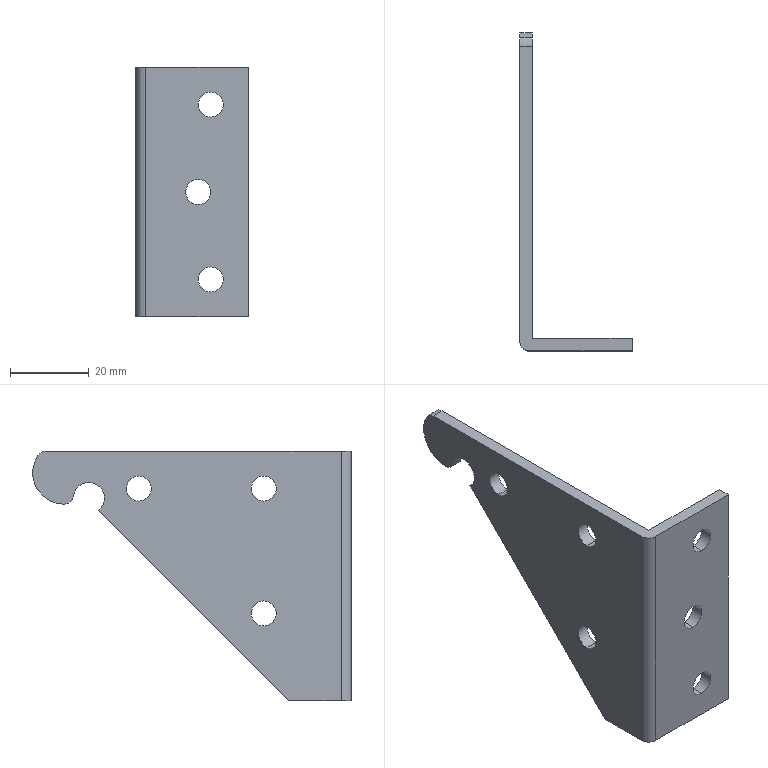Part | SolidWorks | features ICE 3, Extrusion 1 | 1 solid | 26 faces | box 28.575 x 80.975 x 63.5 mm | volume 14204 mm3 | cylinder 18 | plane 8 | commonest cylinder face diameters 6.35 x12 5.08 x4 7.925 x1 15.9 x1
STEP:
#1=CARTESIAN_POINT('',(15.875,0.,-50.8));
#2=VERTEX_POINT('',#1);
#3=CARTESIAN_POINT('',(15.875,0.,-57.15));
#4=VERTEX_POINT('',#3);
#5=CARTESIAN_POINT('',(15.875,0.,-53.975));
#6=DIRECTION('',(0.,-1.,0.));
#7=DIRECTION('',(0.,0.,-1.));
#8=AXIS2_PLACEMENT_3D('',#5,#6,#7);
#9=CIRCLE('',#8,3.175);
#10=EDGE_CURVE('',#2,#4,#9,.T.);
#11=ORIENTED_EDGE('',*,*,#10,.T.);
#12=CARTESIAN_POINT('',(15.875,3.175,-57.15));
#13=VERTEX_POINT('',#12);
#14=CARTESIAN_POINT('',(15.875,-22.225,-57.15));
#15=DIRECTION('',(0.,1.,0.));
#16=VECTOR('',#15,1000.);
#17=LINE('',#14,#16);
#18=EDGE_CURVE('',#4,#13,#17,.T.);
#19=ORIENTED_EDGE('',*,*,#18,.T.);
#20=CARTESIAN_POINT('',(15.875,3.175,-50.8));
#21=VERTEX_POINT('',#20);
#22=CARTESIAN_POINT('',(15.875,3.175,-53.975));
#23=DIRECTION('',(0.,1.,0.));
#24=DIRECTION('',(0.,0.,1.));
#25=AXIS2_PLACEMENT_3D('',#22,#23,#24);
#26=CIRCLE('',#25,3.175);
#27=EDGE_CURVE('',#13,#21,#26,.T.);
#28=ORIENTED_EDGE('',*,*,#27,.T.);
#29=CARTESIAN_POINT('',(15.875,-22.225,-50.8));
#30=DIRECTION('',(0.,1.,0.));
#31=VECTOR('',#30,1000.);
#32=LINE('',#29,#31);
#33=EDGE_CURVE('',#2,#21,#32,.T.);
#34=ORIENTED_EDGE('',*,*,#33,.F.);
#35=EDGE_LOOP('',(#11,#19,#28,#34));
#36=FACE_OUTER_BOUND('',#35,.T.);
#37=CARTESIAN_POINT('',(15.875,-22.225,-53.975));
#38=DIRECTION('',(0.,1.,0.));
#39=DIRECTION('',(0.,0.,1.));
#40=AXIS2_PLACEMENT_3D('',#37,#38,#39);
#41=CYLINDRICAL_SURFACE('',#40,3.175);
#42=ADVANCED_FACE('',(#36),#41,.F.);
#43=CARTESIAN_POINT('',(12.7,0.,-28.575));
#44=VERTEX_POINT('',#43);
#45=CARTESIAN_POINT('',(12.7,0.,-34.925));
#46=VERTEX_POINT('',#45);
#47=CARTESIAN_POINT('',(12.7,0.,-31.75));
#48=DIRECTION('',(0.,-1.,0.));
#49=DIRECTION('',(0.,0.,-1.));
#50=AXIS2_PLACEMENT_3D('',#47,#48,#49);
#51=CIRCLE('',#50,3.175);
#52=EDGE_CURVE('',#44,#46,#51,.T.);
#53=ORIENTED_EDGE('',*,*,#52,.T.);
#54=CARTESIAN_POINT('',(12.7,3.175,-34.925));
#55=VERTEX_POINT('',#54);
#56=CARTESIAN_POINT('',(12.7,-22.225,-34.925));
#57=DIRECTION('',(0.,1.,0.));
#58=VECTOR('',#57,1000.);
#59=LINE('',#56,#58);
#60=EDGE_CURVE('',#46,#55,#59,.T.);
#61=ORIENTED_EDGE('',*,*,#60,.T.);
#62=CARTESIAN_POINT('',(12.7,3.175,-28.575));
#63=VERTEX_POINT('',#62);
#64=CARTESIAN_POINT('',(12.7,3.175,-31.75));
#65=DIRECTION('',(0.,1.,0.));
#66=DIRECTION('',(0.,0.,1.));
#67=AXIS2_PLACEMENT_3D('',#64,#65,#66);
#68=CIRCLE('',#67,3.175);
#69=EDGE_CURVE('',#55,#63,#68,.T.);
#70=ORIENTED_EDGE('',*,*,#69,.T.);
#71=CARTESIAN_POINT('',(12.7,-22.225,-28.575));
#72=DIRECTION('',(0.,1.,0.));
#73=VECTOR('',#72,1000.);
#74=LINE('',#71,#73);
#75=EDGE_CURVE('',#44,#63,#74,.T.);
#76=ORIENTED_EDGE('',*,*,#75,.F.);
#77=EDGE_LOOP('',(#53,#61,#70,#76));
#78=FACE_OUTER_BOUND('',#77,.T.);
#79=CARTESIAN_POINT('',(12.7,-22.225,-31.75));
#80=DIRECTION('',(0.,1.,0.));
#81=DIRECTION('',(0.,0.,1.));
#82=AXIS2_PLACEMENT_3D('',#79,#80,#81);
#83=CYLINDRICAL_SURFACE('',#82,3.175);
#84=ADVANCED_FACE('',(#78),#83,.F.);
#85=CARTESIAN_POINT('',(15.875,0.,-6.35));
#86=VERTEX_POINT('',#85);
#87=CARTESIAN_POINT('',(15.875,0.,-12.7));
#88=VERTEX_POINT('',#87);
#89=CARTESIAN_POINT('',(15.875,0.,-9.525));
#90=DIRECTION('',(0.,-1.,0.));
#91=DIRECTION('',(0.,0.,-1.));
#92=AXIS2_PLACEMENT_3D('',#89,#90,#91);
#93=CIRCLE('',#92,3.175);
#94=EDGE_CURVE('',#86,#88,#93,.T.);
#95=ORIENTED_EDGE('',*,*,#94,.T.);
#96=CARTESIAN_POINT('',(15.875,3.175,-12.7));
#97=VERTEX_POINT('',#96);
#98=CARTESIAN_POINT('',(15.875,-22.225,-12.7));
#99=DIRECTION('',(0.,1.,0.));
#100=VECTOR('',#99,1000.);
#101=LINE('',#98,#100);
#102=EDGE_CURVE('',#88,#97,#101,.T.);
#103=ORIENTED_EDGE('',*,*,#102,.T.);
#104=CARTESIAN_POINT('',(15.875,3.175,-6.35));
#105=VERTEX_POINT('',#104);
#106=CARTESIAN_POINT('',(15.875,3.175,-9.525));
#107=DIRECTION('',(0.,1.,0.));
#108=DIRECTION('',(0.,0.,1.));
#109=AXIS2_PLACEMENT_3D('',#106,#107,#108);
#110=CIRCLE('',#109,3.175);
#111=EDGE_CURVE('',#97,#105,#110,.T.);
#112=ORIENTED_EDGE('',*,*,#111,.T.);
#113=CARTESIAN_POINT('',(15.875,-22.225,-6.35));
#114=DIRECTION('',(0.,1.,0.));
#115=VECTOR('',#114,1000.);
#116=LINE('',#113,#115);
#117=EDGE_CURVE('',#86,#105,#116,.T.);
#118=ORIENTED_EDGE('',*,*,#117,.F.);
#119=EDGE_LOOP('',(#95,#103,#112,#118));
#120=FACE_OUTER_BOUND('',#119,.T.);
#121=CARTESIAN_POINT('',(15.875,-22.225,-9.525));
#122=DIRECTION('',(0.,1.,0.));
#123=DIRECTION('',(0.,0.,1.));
#124=AXIS2_PLACEMENT_3D('',#121,#122,#123);
#125=CYLINDRICAL_SURFACE('',#124,3.175);
#126=ADVANCED_FACE('',(#120),#125,.F.);
#127=CARTESIAN_POINT('',(-3.175,53.975,-6.35));
#128=VERTEX_POINT('',#127);
#129=CARTESIAN_POINT('',(-3.175,53.975,-12.7));
#130=VERTEX_POINT('',#129);
#131=CARTESIAN_POINT('',(-3.175,53.975,-9.525));
#132=DIRECTION('',(1.,0.,0.));
#133=DIRECTION('',(0.,0.,-1.));
#134=AXIS2_PLACEMENT_3D('',#131,#132,#133);
#135=CIRCLE('',#134,3.175);
#136=EDGE_CURVE('',#128,#130,#135,.T.);
#137=ORIENTED_EDGE('',*,*,#136,.F.);
#138=CARTESIAN_POINT('',(0.,53.975,-6.35));
#139=VERTEX_POINT('',#138);
#140=CARTESIAN_POINT('',(-3.175,53.975,-6.35));
#141=DIRECTION('',(1.,0.,0.));
#142=VECTOR('',#141,1000.);
#143=LINE('',#140,#142);
#144=EDGE_CURVE('',#128,#139,#143,.T.);
#145=ORIENTED_EDGE('',*,*,#144,.T.);
#146=CARTESIAN_POINT('',(0.,53.975,-12.7));
#147=VERTEX_POINT('',#146);
#148=CARTESIAN_POINT('',(0.,53.975,-9.525));
#149=DIRECTION('',(1.,0.,0.));
#150=DIRECTION('',(0.,0.,-1.));
#151=AXIS2_PLACEMENT_3D('',#148,#149,#150);
#152=CIRCLE('',#151,3.175);
#153=EDGE_CURVE('',#139,#147,#152,.T.);
#154=ORIENTED_EDGE('',*,*,#153,.T.);
#155=CARTESIAN_POINT('',(-3.175,53.975,-12.7));
#156=DIRECTION('',(1.,0.,0.));
#157=VECTOR('',#156,1000.);
#158=LINE('',#155,#157);
#159=EDGE_CURVE('',#130,#147,#158,.T.);
#160=ORIENTED_EDGE('',*,*,#159,.F.);
#161=EDGE_LOOP('',(#137,#145,#154,#160));
#162=FACE_OUTER_BOUND('',#161,.T.);
#163=CARTESIAN_POINT('',(-3.175,53.975,-9.525));
#164=DIRECTION('',(1.,0.,0.));
#165=DIRECTION('',(0.,0.,-1.));
#166=AXIS2_PLACEMENT_3D('',#163,#164,#165);
#167=CYLINDRICAL_SURFACE('',#166,3.175);
#168=ADVANCED_FACE('',(#162),#167,.F.);
#169=CARTESIAN_POINT('',(-3.175,22.225,-38.1));
#170=VERTEX_POINT('',#169);
#171=CARTESIAN_POINT('',(-3.175,22.225,-44.45));
#172=VERTEX_POINT('',#171);
#173=CARTESIAN_POINT('',(-3.175,22.225,-41.275));
#174=DIRECTION('',(1.,0.,0.));
#175=DIRECTION('',(0.,0.,-1.));
#176=AXIS2_PLACEMENT_3D('',#173,#174,#175);
#177=CIRCLE('',#176,3.175);
#178=EDGE_CURVE('',#170,#172,#177,.T.);
#179=ORIENTED_EDGE('',*,*,#178,.F.);
#180=CARTESIAN_POINT('',(0.,22.225,-38.1));
#181=VERTEX_POINT('',#180);
#182=CARTESIAN_POINT('',(-3.175,22.225,-38.1));
#183=DIRECTION('',(1.,0.,0.));
#184=VECTOR('',#183,1000.);
#185=LINE('',#182,#184);
#186=EDGE_CURVE('',#170,#181,#185,.T.);
#187=ORIENTED_EDGE('',*,*,#186,.T.);
#188=CARTESIAN_POINT('',(0.,22.225,-44.45));
#189=VERTEX_POINT('',#188);
#190=CARTESIAN_POINT('',(0.,22.225,-41.275));
#191=DIRECTION('',(1.,0.,0.));
#192=DIRECTION('',(0.,0.,-1.));
#193=AXIS2_PLACEMENT_3D('',#190,#191,#192);
#194=CIRCLE('',#193,3.175);
#195=EDGE_CURVE('',#181,#189,#194,.T.);
#196=ORIENTED_EDGE('',*,*,#195,.T.);
#197=CARTESIAN_POINT('',(-3.175,22.225,-44.45));
#198=DIRECTION('',(1.,0.,0.));
#199=VECTOR('',#198,1000.);
#200=LINE('',#197,#199);
#201=EDGE_CURVE('',#172,#189,#200,.T.);
#202=ORIENTED_EDGE('',*,*,#201,.F.);
#203=EDGE_LOOP('',(#179,#187,#196,#202));
#204=FACE_OUTER_BOUND('',#203,.T.);
#205=CARTESIAN_POINT('',(-3.175,22.225,-41.275));
#206=DIRECTION('',(1.,0.,0.));
#207=DIRECTION('',(0.,0.,-1.));
#208=AXIS2_PLACEMENT_3D('',#205,#206,#207);
#209=CYLINDRICAL_SURFACE('',#208,3.175);
#210=ADVANCED_FACE('',(#204),#209,.F.);
#211=CARTESIAN_POINT('',(-3.175,22.225,-6.35));
#212=VERTEX_POINT('',#211);
#213=CARTESIAN_POINT('',(-3.175,22.225,-12.7));
#214=VERTEX_POINT('',#213);
#215=CARTESIAN_POINT('',(-3.175,22.225,-9.525));
#216=DIRECTION('',(1.,0.,0.));
#217=DIRECTION('',(0.,0.,-1.));
#218=AXIS2_PLACEMENT_3D('',#215,#216,#217);
#219=CIRCLE('',#218,3.175);
#220=EDGE_CURVE('',#212,#214,#219,.T.);
#221=ORIENTED_EDGE('',*,*,#220,.F.);
#222=CARTESIAN_POINT('',(0.,22.225,-6.35));
#223=VERTEX_POINT('',#222);
#224=CARTESIAN_POINT('',(-3.175,22.225,-6.35));
#225=DIRECTION('',(1.,0.,0.));
#226=VECTOR('',#225,1000.);
#227=LINE('',#224,#226);
#228=EDGE_CURVE('',#212,#223,#227,.T.);
#229=ORIENTED_EDGE('',*,*,#228,.T.);
#230=CARTESIAN_POINT('',(0.,22.225,-12.7));
#231=VERTEX_POINT('',#230);
#232=CARTESIAN_POINT('',(0.,22.225,-9.525));
#233=DIRECTION('',(1.,0.,0.));
#234=DIRECTION('',(0.,0.,-1.));
#235=AXIS2_PLACEMENT_3D('',#232,#233,#234);
#236=CIRCLE('',#235,3.175);
#237=EDGE_CURVE('',#223,#231,#236,.T.);
#238=ORIENTED_EDGE('',*,*,#237,.T.);
#239=CARTESIAN_POINT('',(-3.175,22.225,-12.7));
#240=DIRECTION('',(1.,0.,0.));
#241=VECTOR('',#240,1000.);
#242=LINE('',#239,#241);
#243=EDGE_CURVE('',#214,#231,#242,.T.);
#244=ORIENTED_EDGE('',*,*,#243,.F.);
#245=EDGE_LOOP('',(#221,#229,#238,#244));
#246=FACE_OUTER_BOUND('',#245,.T.);
#247=CARTESIAN_POINT('',(-3.175,22.225,-9.525));
#248=DIRECTION('',(1.,0.,0.));
#249=DIRECTION('',(0.,0.,-1.));
#250=AXIS2_PLACEMENT_3D('',#247,#248,#249);
#251=CYLINDRICAL_SURFACE('',#250,3.175);
#252=ADVANCED_FACE('',(#246),#251,.F.);
#253=CARTESIAN_POINT('',(-3.175,73.109,-13.512));
#254=VERTEX_POINT('',#253);
#255=CARTESIAN_POINT('',(-3.175,70.596,-11.34));
#256=VERTEX_POINT('',#255);
#257=CARTESIAN_POINT('',(-3.175,73.109,-10.972));
#258=DIRECTION('',(-1.,0.,0.));
#259=DIRECTION('',(0.,0.,-1.));
#260=AXIS2_PLACEMENT_3D('',#257,#258,#259);
#261=CIRCLE('',#260,2.54);
#262=EDGE_CURVE('',#254,#256,#261,.T.);
#263=ORIENTED_EDGE('',*,*,#262,.F.);
#264=CARTESIAN_POINT('',(0.,73.109,-13.512));
#265=VERTEX_POINT('',#264);
#266=CARTESIAN_POINT('',(-3.175,73.109,-13.512));
#267=DIRECTION('',(1.,0.,0.));
#268=VECTOR('',#267,1000.);
#269=LINE('',#266,#268);
#270=EDGE_CURVE('',#254,#265,#269,.T.);
#271=ORIENTED_EDGE('',*,*,#270,.T.);
#272=CARTESIAN_POINT('',(0.,70.596,-11.34));
#273=VERTEX_POINT('',#272);
#274=CARTESIAN_POINT('',(0.,73.109,-10.972));
#275=DIRECTION('',(-1.,0.,0.));
#276=DIRECTION('',(0.,0.,-1.));
#277=AXIS2_PLACEMENT_3D('',#274,#275,#276);
#278=CIRCLE('',#277,2.54);
#279=EDGE_CURVE('',#265,#273,#278,.T.);
#280=ORIENTED_EDGE('',*,*,#279,.T.);
#281=CARTESIAN_POINT('',(-3.175,70.596,-11.34));
#282=DIRECTION('',(1.,0.,0.));
#283=VECTOR('',#282,1000.);
#284=LINE('',#281,#283);
#285=EDGE_CURVE('',#256,#273,#284,.T.);
#286=ORIENTED_EDGE('',*,*,#285,.F.);
#287=EDGE_LOOP('',(#263,#271,#280,#286));
#288=FACE_OUTER_BOUND('',#287,.T.);
#289=CARTESIAN_POINT('',(-3.175,73.109,-10.972));
#290=DIRECTION('',(1.,0.,0.));
#291=DIRECTION('',(0.,0.,-1.));
#292=AXIS2_PLACEMENT_3D('',#289,#290,#291);
#293=CYLINDRICAL_SURFACE('',#292,2.54);
#294=ADVANCED_FACE('',(#288),#293,.T.);
#295=CARTESIAN_POINT('',(-0.635,0.,-63.5));
#296=VERTEX_POINT('',#295);
#297=CARTESIAN_POINT('',(-3.175,2.54,-63.5));
#298=VERTEX_POINT('',#297);
#299=CARTESIAN_POINT('',(-0.635,2.54,-63.5));
#300=DIRECTION('',(0.,0.,-1.));
#301=DIRECTION('',(1.,0.,0.));
#302=AXIS2_PLACEMENT_3D('',#299,#300,#301);
#303=CIRCLE('',#302,2.54);
#304=EDGE_CURVE('',#296,#298,#303,.T.);
#305=ORIENTED_EDGE('',*,*,#304,.T.);
#306=CARTESIAN_POINT('',(-3.175,15.875,-63.5));
#307=VERTEX_POINT('',#306);
#308=CARTESIAN_POINT('',(-3.175,0.,-63.5));
#309=DIRECTION('',(0.,1.,0.));
#310=VECTOR('',#309,1000.);
#311=LINE('',#308,#310);
#312=EDGE_CURVE('',#298,#307,#311,.T.);
#313=ORIENTED_EDGE('',*,*,#312,.T.);
#314=CARTESIAN_POINT('',(0.,15.875,-63.5));
#315=VERTEX_POINT('',#314);
#316=CARTESIAN_POINT('',(-3.175,15.875,-63.5));
#317=DIRECTION('',(1.,0.,0.));
#318=VECTOR('',#317,1000.);
#319=LINE('',#316,#318);
#320=EDGE_CURVE('',#307,#315,#319,.T.);
#321=ORIENTED_EDGE('',*,*,#320,.T.);
#322=CARTESIAN_POINT('',(0.,3.175,-63.5));
#323=VERTEX_POINT('',#322);
#324=CARTESIAN_POINT('',(0.,0.,-63.5));
#325=DIRECTION('',(0.,1.,0.));
#326=VECTOR('',#325,1000.);
#327=LINE('',#324,#326);
#328=EDGE_CURVE('',#323,#315,#327,.T.);
#329=ORIENTED_EDGE('',*,*,#328,.F.);
#330=CARTESIAN_POINT('',(25.4,3.175,-63.5));
#331=VERTEX_POINT('',#330);
#332=CARTESIAN_POINT('',(25.4,3.175,-63.5));
#333=DIRECTION('',(-1.,0.,0.));
#334=VECTOR('',#333,1000.);
#335=LINE('',#332,#334);
#336=EDGE_CURVE('',#331,#323,#335,.T.);
#337=ORIENTED_EDGE('',*,*,#336,.F.);
#338=CARTESIAN_POINT('',(25.4,0.,-63.5));
#339=VERTEX_POINT('',#338);
#340=CARTESIAN_POINT('',(25.4,0.,-63.5));
#341=DIRECTION('',(0.,1.,0.));
#342=VECTOR('',#341,1000.);
#343=LINE('',#340,#342);
#344=EDGE_CURVE('',#339,#331,#343,.T.);
#345=ORIENTED_EDGE('',*,*,#344,.F.);
#346=CARTESIAN_POINT('',(-3.175,0.,-63.5));
#347=DIRECTION('',(1.,0.,0.));
#348=VECTOR('',#347,1000.);
#349=LINE('',#346,#348);
#350=EDGE_CURVE('',#296,#339,#349,.T.);
#351=ORIENTED_EDGE('',*,*,#350,.F.);
#352=EDGE_LOOP('',(#305,#313,#321,#329,#337,#345,#351));
#353=FACE_OUTER_BOUND('',#352,.T.);
#354=CARTESIAN_POINT('',(-3.175,0.,-63.5));
#355=DIRECTION('',(0.,0.,-1.));
#356=DIRECTION('',(-1.,0.,0.));
#357=AXIS2_PLACEMENT_3D('',#354,#355,#356);
#358=PLANE('',#357);
#359=ADVANCED_FACE('',(#353),#358,.T.);
#360=ORIENTED_EDGE('',*,*,#10,.F.);
#361=CARTESIAN_POINT('',(15.875,0.,-53.975));
#362=DIRECTION('',(0.,-1.,0.));
#363=DIRECTION('',(0.,0.,-1.));
#364=AXIS2_PLACEMENT_3D('',#361,#362,#363);
#365=CIRCLE('',#364,3.175);
#366=EDGE_CURVE('',#4,#2,#365,.T.);
#367=ORIENTED_EDGE('',*,*,#366,.F.);
#368=EDGE_LOOP('',(#360,#367));
#369=FACE_BOUND('',#368,.T.);
#370=ORIENTED_EDGE('',*,*,#52,.F.);
#371=CARTESIAN_POINT('',(12.7,0.,-31.75));
#372=DIRECTION('',(0.,-1.,0.));
#373=DIRECTION('',(0.,0.,-1.));
#374=AXIS2_PLACEMENT_3D('',#371,#372,#373);
#375=CIRCLE('',#374,3.175);
#376=EDGE_CURVE('',#46,#44,#375,.T.);
#377=ORIENTED_EDGE('',*,*,#376,.F.);
#378=EDGE_LOOP('',(#370,#377));
#379=FACE_BOUND('',#378,.T.);
#380=ORIENTED_EDGE('',*,*,#94,.F.);
#381=CARTESIAN_POINT('',(15.875,0.,-9.525));
#382=DIRECTION('',(0.,-1.,0.));
#383=DIRECTION('',(0.,0.,-1.));
#384=AXIS2_PLACEMENT_3D('',#381,#382,#383);
#385=CIRCLE('',#384,3.175);
#386=EDGE_CURVE('',#88,#86,#385,.T.);
#387=ORIENTED_EDGE('',*,*,#386,.F.);
#388=EDGE_LOOP('',(#380,#387));
#389=FACE_BOUND('',#388,.T.);
#390=CARTESIAN_POINT('',(-0.635,0.,0.));
#391=VERTEX_POINT('',#390);
#392=CARTESIAN_POINT('',(25.4,0.,0.));
#393=VERTEX_POINT('',#392);
#394=CARTESIAN_POINT('',(-3.175,0.,0.));
#395=DIRECTION('',(1.,0.,0.));
#396=VECTOR('',#395,1000.);
#397=LINE('',#394,#396);
#398=EDGE_CURVE('',#391,#393,#397,.T.);
#399=ORIENTED_EDGE('',*,*,#398,.F.);
#400=CARTESIAN_POINT('',(-0.635,0.,-63.5));
#401=DIRECTION('',(0.,0.,1.));
#402=VECTOR('',#401,1000.);
#403=LINE('',#400,#402);
#404=EDGE_CURVE('',#296,#391,#403,.T.);
#405=ORIENTED_EDGE('',*,*,#404,.F.);
#406=ORIENTED_EDGE('',*,*,#350,.T.);
#407=CARTESIAN_POINT('',(25.4,0.,0.));
#408=DIRECTION('',(0.,0.,-1.));
#409=VECTOR('',#408,1000.);
#410=LINE('',#407,#409);
#411=EDGE_CURVE('',#393,#339,#410,.T.);
#412=ORIENTED_EDGE('',*,*,#411,.F.);
#413=EDGE_LOOP('',(#399,#405,#406,#412));
#414=FACE_OUTER_BOUND('',#413,.T.);
#415=CARTESIAN_POINT('',(-3.175,0.,0.));
#416=DIRECTION('',(0.,-1.,0.));
#417=DIRECTION('',(0.,0.,-1.));
#418=AXIS2_PLACEMENT_3D('',#415,#416,#417);
#419=PLANE('',#418);
#420=ADVANCED_FACE('',(#369,#379,#389,#414),#419,.T.);
#421=CARTESIAN_POINT('',(-3.175,2.54,0.));
#422=VERTEX_POINT('',#421);
#423=CARTESIAN_POINT('',(-0.635,2.54,0.));
#424=DIRECTION('',(0.,0.,-1.));
#425=DIRECTION('',(1.,0.,0.));
#426=AXIS2_PLACEMENT_3D('',#423,#424,#425);
#427=CIRCLE('',#426,2.54);
#428=EDGE_CURVE('',#391,#422,#427,.T.);
#429=ORIENTED_EDGE('',*,*,#428,.F.);
#430=ORIENTED_EDGE('',*,*,#398,.T.);
#431=CARTESIAN_POINT('',(25.4,3.175,0.));
#432=VERTEX_POINT('',#431);
#433=CARTESIAN_POINT('',(25.4,0.,0.));
#434=DIRECTION('',(0.,-1.,0.));
#435=VECTOR('',#434,1000.);
#436=LINE('',#433,#435);
#437=EDGE_CURVE('',#432,#393,#436,.T.);
#438=ORIENTED_EDGE('',*,*,#437,.F.);
#439=CARTESIAN_POINT('',(0.,3.175,0.));
#440=VERTEX_POINT('',#439);
#441=CARTESIAN_POINT('',(25.4,3.175,0.));
#442=DIRECTION('',(-1.,0.,0.));
#443=VECTOR('',#442,1000.);
#444=LINE('',#441,#443);
#445=EDGE_CURVE('',#432,#440,#444,.T.);
#446=ORIENTED_EDGE('',*,*,#445,.T.);
#447=CARTESIAN_POINT('',(0.,77.512,0.));
#448=VERTEX_POINT('',#447);
#449=CARTESIAN_POINT('',(0.,0.,0.));
#450=DIRECTION('',(0.,-1.,0.));
#451=VECTOR('',#450,1000.);
#452=LINE('',#449,#451);
#453=EDGE_CURVE('',#448,#440,#452,.T.);
#454=ORIENTED_EDGE('',*,*,#453,.F.);
#455=CARTESIAN_POINT('',(-3.175,77.512,0.));
#456=VERTEX_POINT('',#455);
#457=CARTESIAN_POINT('',(-3.175,77.512,0.));
#458=DIRECTION('',(1.,0.,0.));
#459=VECTOR('',#458,1000.);
#460=LINE('',#457,#459);
#461=EDGE_CURVE('',#456,#448,#460,.T.);
#462=ORIENTED_EDGE('',*,*,#461,.F.);
#463=CARTESIAN_POINT('',(-3.175,0.,0.));
#464=DIRECTION('',(0.,-1.,0.));
#465=VECTOR('',#464,1000.);
#466=LINE('',#463,#465);
#467=EDGE_CURVE('',#456,#422,#466,.T.);
#468=ORIENTED_EDGE('',*,*,#467,.T.);
#469=EDGE_LOOP('',(#429,#430,#438,#446,#454,#462,#468));
#470=FACE_OUTER_BOUND('',#469,.T.);
#471=CARTESIAN_POINT('',(-3.175,0.,0.));
#472=DIRECTION('',(0.,0.,1.));
#473=DIRECTION('',(1.,0.,0.));
#474=AXIS2_PLACEMENT_3D('',#471,#472,#473);
#475=PLANE('',#474);
#476=ADVANCED_FACE('',(#470),#475,.T.);
#477=CARTESIAN_POINT('',(-3.175,53.975,-9.525));
#478=DIRECTION('',(1.,0.,0.));
#479=DIRECTION('',(0.,0.,-1.));
#480=AXIS2_PLACEMENT_3D('',#477,#478,#479);
#481=CIRCLE('',#480,3.175);
#482=EDGE_CURVE('',#130,#128,#481,.T.);
#483=ORIENTED_EDGE('',*,*,#482,.T.);
#484=ORIENTED_EDGE('',*,*,#136,.T.);
#485=EDGE_LOOP('',(#483,#484));
#486=FACE_BOUND('',#485,.T.);
#487=CARTESIAN_POINT('',(-3.175,22.225,-9.525));
#488=DIRECTION('',(1.,0.,0.));
#489=DIRECTION('',(0.,0.,-1.));
#490=AXIS2_PLACEMENT_3D('',#487,#488,#489);
#491=CIRCLE('',#490,3.175);
#492=EDGE_CURVE('',#214,#212,#491,.T.);
#493=ORIENTED_EDGE('',*,*,#492,.T.);
#494=ORIENTED_EDGE('',*,*,#220,.T.);
#495=EDGE_LOOP('',(#493,#494));
#496=FACE_BOUND('',#495,.T.);
#497=CARTESIAN_POINT('',(-3.175,22.225,-41.275));
#498=DIRECTION('',(1.,0.,0.));
#499=DIRECTION('',(0.,0.,-1.));
#500=AXIS2_PLACEMENT_3D('',#497,#498,#499);
#501=CIRCLE('',#500,3.175);
#502=EDGE_CURVE('',#172,#170,#501,.T.);
#503=ORIENTED_EDGE('',*,*,#502,.T.);
#504=ORIENTED_EDGE('',*,*,#178,.T.);
#505=EDGE_LOOP('',(#503,#504));
#506=FACE_BOUND('',#505,.T.);
#507=CARTESIAN_POINT('',(-3.175,2.54,-63.5));
#508=DIRECTION('',(0.,0.,1.));
#509=VECTOR('',#508,1000.);
#510=LINE('',#507,#509);
#511=EDGE_CURVE('',#298,#422,#510,.T.);
#512=ORIENTED_EDGE('',*,*,#511,.T.);
#513=ORIENTED_EDGE('',*,*,#467,.F.);
#514=CARTESIAN_POINT('',(-3.175,79.619,-1.121));
#515=VERTEX_POINT('',#514);
#516=CARTESIAN_POINT('',(-3.175,77.512,-2.54));
#517=DIRECTION('',(-1.,0.,0.));
#518=DIRECTION('',(0.,0.,-1.));
#519=AXIS2_PLACEMENT_3D('',#516,#517,#518);
#520=CIRCLE('',#519,2.54);
#521=EDGE_CURVE('',#456,#515,#520,.T.);
#522=ORIENTED_EDGE('',*,*,#521,.T.);
#523=CARTESIAN_POINT('',(-3.175,73.148,-13.512));
#524=VERTEX_POINT('',#523);
#525=CARTESIAN_POINT('',(-3.175,73.025,-5.563));
#526=DIRECTION('',(-1.,0.,0.));
#527=DIRECTION('',(0.,0.,-1.));
#528=AXIS2_PLACEMENT_3D('',#525,#526,#527);
#529=CIRCLE('',#528,7.95);
#530=EDGE_CURVE('',#515,#524,#529,.T.);
#531=ORIENTED_EDGE('',*,*,#530,.T.);
#532=CARTESIAN_POINT('',(-3.175,73.109,-10.972));
#533=DIRECTION('',(-1.,0.,0.));
#534=DIRECTION('',(0.,0.,-1.));
#535=AXIS2_PLACEMENT_3D('',#532,#533,#534);
#536=CIRCLE('',#535,2.54);
#537=EDGE_CURVE('',#524,#254,#536,.T.);
#538=ORIENTED_EDGE('',*,*,#537,.T.);
#539=ORIENTED_EDGE('',*,*,#262,.T.);
#540=CARTESIAN_POINT('',(-3.175,64.295,-15.08));
#541=VERTEX_POINT('',#540);
#542=CARTESIAN_POINT('',(-3.175,66.675,-11.913));
#543=DIRECTION('',(-1.,0.,0.));
#544=DIRECTION('',(0.,0.,-1.));
#545=AXIS2_PLACEMENT_3D('',#542,#543,#544);
#546=CIRCLE('',#545,3.962);
#547=EDGE_CURVE('',#541,#256,#546,.T.);
#548=ORIENTED_EDGE('',*,*,#547,.F.);
#549=CARTESIAN_POINT('',(-3.175,39.688,-39.687));
#550=DIRECTION('',(0.,0.7071,0.7071));
#551=VECTOR('',#550,1000.);
#552=LINE('',#549,#551);
#553=EDGE_CURVE('',#307,#541,#552,.T.);
#554=ORIENTED_EDGE('',*,*,#553,.F.);
#555=ORIENTED_EDGE('',*,*,#312,.F.);
#556=EDGE_LOOP('',(#512,#513,#522,#531,#538,#539,#548,#554,#555));
#557=FACE_OUTER_BOUND('',#556,.T.);
#558=CARTESIAN_POINT('',(-3.175,0.,0.));
#559=DIRECTION('',(1.,0.,0.));
#560=DIRECTION('',(0.,0.,-1.));
#561=AXIS2_PLACEMENT_3D('',#558,#559,#560);
#562=PLANE('',#561);
#563=ADVANCED_FACE('',(#486,#496,#506,#557),#562,.F.);
#564=CARTESIAN_POINT('',(0.,79.619,-1.121));
#565=VERTEX_POINT('',#564);
#566=CARTESIAN_POINT('',(0.,77.512,-2.54));
#567=DIRECTION('',(-1.,0.,0.));
#568=DIRECTION('',(0.,0.,-1.));
#569=AXIS2_PLACEMENT_3D('',#566,#567,#568);
#570=CIRCLE('',#569,2.54);
#571=EDGE_CURVE('',#448,#565,#570,.T.);
#572=ORIENTED_EDGE('',*,*,#571,.T.);
#573=CARTESIAN_POINT('',(-3.175,79.619,-1.121));
#574=DIRECTION('',(1.,0.,0.));
#575=VECTOR('',#574,1000.);
#576=LINE('',#573,#575);
#577=EDGE_CURVE('',#515,#565,#576,.T.);
#578=ORIENTED_EDGE('',*,*,#577,.F.);
#579=ORIENTED_EDGE('',*,*,#521,.F.);
#580=ORIENTED_EDGE('',*,*,#461,.T.);
#581=EDGE_LOOP('',(#572,#578,#579,#580));
#582=FACE_OUTER_BOUND('',#581,.T.);
#583=CARTESIAN_POINT('',(-3.175,77.512,-2.54));
#584=DIRECTION('',(1.,0.,0.));
#585=DIRECTION('',(0.,0.,-1.));
#586=AXIS2_PLACEMENT_3D('',#583,#584,#585);
#587=CYLINDRICAL_SURFACE('',#586,2.54);
#588=ADVANCED_FACE('',(#582),#587,.T.);
#589=CARTESIAN_POINT('',(0.,73.148,-13.512));
#590=VERTEX_POINT('',#589);
#591=CARTESIAN_POINT('',(0.,73.025,-5.563));
#592=DIRECTION('',(-1.,0.,0.));
#593=DIRECTION('',(0.,0.,-1.));
#594=AXIS2_PLACEMENT_3D('',#591,#592,#593);
#595=CIRCLE('',#594,7.95);
#596=EDGE_CURVE('',#565,#590,#595,.T.);
#597=ORIENTED_EDGE('',*,*,#596,.T.);
#598=CARTESIAN_POINT('',(-3.175,73.148,-13.512));
#599=DIRECTION('',(1.,0.,0.));
#600=VECTOR('',#599,1000.);
#601=LINE('',#598,#600);
#602=EDGE_CURVE('',#524,#590,#601,.T.);
#603=ORIENTED_EDGE('',*,*,#602,.F.);
#604=ORIENTED_EDGE('',*,*,#530,.F.);
#605=ORIENTED_EDGE('',*,*,#577,.T.);
#606=EDGE_LOOP('',(#597,#603,#604,#605));
#607=FACE_OUTER_BOUND('',#606,.T.);
#608=CARTESIAN_POINT('',(-3.175,73.025,-5.563));
#609=DIRECTION('',(1.,0.,0.));
#610=DIRECTION('',(0.,0.,-1.));
#611=AXIS2_PLACEMENT_3D('',#608,#609,#610);
#612=CYLINDRICAL_SURFACE('',#611,7.95);
#613=ADVANCED_FACE('',(#607),#612,.T.);
#614=ORIENTED_EDGE('',*,*,#270,.F.);
#615=ORIENTED_EDGE('',*,*,#537,.F.);
#616=ORIENTED_EDGE('',*,*,#602,.T.);
#617=CARTESIAN_POINT('',(0.,73.109,-10.972));
#618=DIRECTION('',(-1.,0.,0.));
#619=DIRECTION('',(0.,0.,-1.));
#620=AXIS2_PLACEMENT_3D('',#617,#618,#619);
#621=CIRCLE('',#620,2.54);
#622=EDGE_CURVE('',#590,#265,#621,.T.);
#623=ORIENTED_EDGE('',*,*,#622,.T.);
#624=EDGE_LOOP('',(#614,#615,#616,#623));
#625=FACE_OUTER_BOUND('',#624,.T.);
#626=CARTESIAN_POINT('',(-3.175,73.109,-10.972));
#627=DIRECTION('',(1.,0.,0.));
#628=DIRECTION('',(0.,0.,-1.));
#629=AXIS2_PLACEMENT_3D('',#626,#627,#628);
#630=CYLINDRICAL_SURFACE('',#629,2.54);
#631=ADVANCED_FACE('',(#625),#630,.T.);
#632=CARTESIAN_POINT('',(0.,64.295,-15.08));
#633=VERTEX_POINT('',#632);
#634=CARTESIAN_POINT('',(0.,66.675,-11.913));
#635=DIRECTION('',(-1.,0.,0.));
#636=DIRECTION('',(0.,0.,-1.));
#637=AXIS2_PLACEMENT_3D('',#634,#635,#636);
#638=CIRCLE('',#637,3.962);
#639=EDGE_CURVE('',#633,#273,#638,.T.);
#640=ORIENTED_EDGE('',*,*,#639,.F.);
#641=CARTESIAN_POINT('',(-3.175,64.295,-15.08));
#642=DIRECTION('',(1.,0.,0.));
#643=VECTOR('',#642,1000.);
#644=LINE('',#641,#643);
#645=EDGE_CURVE('',#541,#633,#644,.T.);
#646=ORIENTED_EDGE('',*,*,#645,.F.);
#647=ORIENTED_EDGE('',*,*,#547,.T.);
#648=ORIENTED_EDGE('',*,*,#285,.T.);
#649=EDGE_LOOP('',(#640,#646,#647,#648));
#650=FACE_OUTER_BOUND('',#649,.T.);
#651=CARTESIAN_POINT('',(-3.175,66.675,-11.913));
#652=DIRECTION('',(1.,0.,0.));
#653=DIRECTION('',(0.,0.,-1.));
#654=AXIS2_PLACEMENT_3D('',#651,#652,#653);
#655=CYLINDRICAL_SURFACE('',#654,3.962);
#656=ADVANCED_FACE('',(#650),#655,.F.);
#657=CARTESIAN_POINT('',(0.,39.688,-39.687));
#658=DIRECTION('',(0.,0.7071,0.7071));
#659=VECTOR('',#658,1000.);
#660=LINE('',#657,#659);
#661=EDGE_CURVE('',#315,#633,#660,.T.);
#662=ORIENTED_EDGE('',*,*,#661,.F.);
#663=ORIENTED_EDGE('',*,*,#320,.F.);
#664=ORIENTED_EDGE('',*,*,#553,.T.);
#665=ORIENTED_EDGE('',*,*,#645,.T.);
#666=EDGE_LOOP('',(#662,#663,#664,#665));
#667=FACE_OUTER_BOUND('',#666,.T.);
#668=CARTESIAN_POINT('',(-3.175,39.688,-39.687));
#669=DIRECTION('',(0.,0.7071,-0.7071));
#670=DIRECTION('',(0.,0.7071,0.7071));
#671=AXIS2_PLACEMENT_3D('',#668,#669,#670);
#672=PLANE('',#671);
#673=ADVANCED_FACE('',(#667),#672,.T.);
#674=ORIENTED_EDGE('',*,*,#228,.F.);
#675=ORIENTED_EDGE('',*,*,#492,.F.);
#676=ORIENTED_EDGE('',*,*,#243,.T.);
#677=CARTESIAN_POINT('',(0.,22.225,-9.525));
#678=DIRECTION('',(1.,0.,0.));
#679=DIRECTION('',(0.,0.,-1.));
#680=AXIS2_PLACEMENT_3D('',#677,#678,#679);
#681=CIRCLE('',#680,3.175);
#682=EDGE_CURVE('',#231,#223,#681,.T.);
#683=ORIENTED_EDGE('',*,*,#682,.T.);
#684=EDGE_LOOP('',(#674,#675,#676,#683));
#685=FACE_OUTER_BOUND('',#684,.T.);
#686=CARTESIAN_POINT('',(-3.175,22.225,-9.525));
#687=DIRECTION('',(1.,0.,0.));
#688=DIRECTION('',(0.,0.,-1.));
#689=AXIS2_PLACEMENT_3D('',#686,#687,#688);
#690=CYLINDRICAL_SURFACE('',#689,3.175);
#691=ADVANCED_FACE('',(#685),#690,.F.);
#692=ORIENTED_EDGE('',*,*,#186,.F.);
#693=ORIENTED_EDGE('',*,*,#502,.F.);
#694=ORIENTED_EDGE('',*,*,#201,.T.);
#695=CARTESIAN_POINT('',(0.,22.225,-41.275));
#696=DIRECTION('',(1.,0.,0.));
#697=DIRECTION('',(0.,0.,-1.));
#698=AXIS2_PLACEMENT_3D('',#695,#696,#697);
#699=CIRCLE('',#698,3.175);
#700=EDGE_CURVE('',#189,#181,#699,.T.);
#701=ORIENTED_EDGE('',*,*,#700,.T.);
#702=EDGE_LOOP('',(#692,#693,#694,#701));
#703=FACE_OUTER_BOUND('',#702,.T.);
#704=CARTESIAN_POINT('',(-3.175,22.225,-41.275));
#705=DIRECTION('',(1.,0.,0.));
#706=DIRECTION('',(0.,0.,-1.));
#707=AXIS2_PLACEMENT_3D('',#704,#705,#706);
#708=CYLINDRICAL_SURFACE('',#707,3.175);
#709=ADVANCED_FACE('',(#703),#708,.F.);
#710=ORIENTED_EDGE('',*,*,#144,.F.);
#711=ORIENTED_EDGE('',*,*,#482,.F.);
#712=ORIENTED_EDGE('',*,*,#159,.T.);
#713=CARTESIAN_POINT('',(0.,53.975,-9.525));
#714=DIRECTION('',(1.,0.,0.));
#715=DIRECTION('',(0.,0.,-1.));
#716=AXIS2_PLACEMENT_3D('',#713,#714,#715);
#717=CIRCLE('',#716,3.175);
#718=EDGE_CURVE('',#147,#139,#717,.T.);
#719=ORIENTED_EDGE('',*,*,#718,.T.);
#720=EDGE_LOOP('',(#710,#711,#712,#719));
#721=FACE_OUTER_BOUND('',#720,.T.);
#722=CARTESIAN_POINT('',(-3.175,53.975,-9.525));
#723=DIRECTION('',(1.,0.,0.));
#724=DIRECTION('',(0.,0.,-1.));
#725=AXIS2_PLACEMENT_3D('',#722,#723,#724);
#726=CYLINDRICAL_SURFACE('',#725,3.175);
#727=ADVANCED_FACE('',(#721),#726,.F.);
#728=CARTESIAN_POINT('',(0.,3.175,0.));
#729=DIRECTION('',(0.,0.,1.));
#730=VECTOR('',#729,1000.);
#731=LINE('',#728,#730);
#732=EDGE_CURVE('',#323,#440,#731,.T.);
#733=ORIENTED_EDGE('',*,*,#732,.F.);
#734=ORIENTED_EDGE('',*,*,#328,.T.);
#735=ORIENTED_EDGE('',*,*,#661,.T.);
#736=ORIENTED_EDGE('',*,*,#639,.T.);
#737=ORIENTED_EDGE('',*,*,#279,.F.);
#738=ORIENTED_EDGE('',*,*,#622,.F.);
#739=ORIENTED_EDGE('',*,*,#596,.F.);
#740=ORIENTED_EDGE('',*,*,#571,.F.);
#741=ORIENTED_EDGE('',*,*,#453,.T.);
#742=EDGE_LOOP('',(#733,#734,#735,#736,#737,#738,#739,#740,#741));
#743=FACE_OUTER_BOUND('',#742,.T.);
#744=ORIENTED_EDGE('',*,*,#700,.F.);
#745=ORIENTED_EDGE('',*,*,#195,.F.);
#746=EDGE_LOOP('',(#744,#745));
#747=FACE_BOUND('',#746,.T.);
#748=ORIENTED_EDGE('',*,*,#682,.F.);
#749=ORIENTED_EDGE('',*,*,#237,.F.);
#750=EDGE_LOOP('',(#748,#749));
#751=FACE_BOUND('',#750,.T.);
#752=ORIENTED_EDGE('',*,*,#718,.F.);
#753=ORIENTED_EDGE('',*,*,#153,.F.);
#754=EDGE_LOOP('',(#752,#753));
#755=FACE_BOUND('',#754,.T.);
#756=CARTESIAN_POINT('',(0.,0.,0.));
#757=DIRECTION('',(1.,0.,0.));
#758=DIRECTION('',(0.,0.,-1.));
#759=AXIS2_PLACEMENT_3D('',#756,#757,#758);
#760=PLANE('',#759);
#761=ADVANCED_FACE('',(#743,#747,#751,#755),#760,.T.);
#762=CARTESIAN_POINT('',(15.875,3.175,-53.975));
#763=DIRECTION('',(0.,1.,0.));
#764=DIRECTION('',(0.,0.,1.));
#765=AXIS2_PLACEMENT_3D('',#762,#763,#764);
#766=CIRCLE('',#765,3.175);
#767=EDGE_CURVE('',#21,#13,#766,.T.);
#768=ORIENTED_EDGE('',*,*,#767,.F.);
#769=ORIENTED_EDGE('',*,*,#27,.F.);
#770=EDGE_LOOP('',(#768,#769));
#771=FACE_BOUND('',#770,.T.);
#772=CARTESIAN_POINT('',(12.7,3.175,-31.75));
#773=DIRECTION('',(0.,1.,0.));
#774=DIRECTION('',(0.,0.,1.));
#775=AXIS2_PLACEMENT_3D('',#772,#773,#774);
#776=CIRCLE('',#775,3.175);
#777=EDGE_CURVE('',#63,#55,#776,.T.);
#778=ORIENTED_EDGE('',*,*,#777,.F.);
#779=ORIENTED_EDGE('',*,*,#69,.F.);
#780=EDGE_LOOP('',(#778,#779));
#781=FACE_BOUND('',#780,.T.);
#782=CARTESIAN_POINT('',(15.875,3.175,-9.525));
#783=DIRECTION('',(0.,1.,0.));
#784=DIRECTION('',(0.,0.,1.));
#785=AXIS2_PLACEMENT_3D('',#782,#783,#784);
#786=CIRCLE('',#785,3.175);
#787=EDGE_CURVE('',#105,#97,#786,.T.);
#788=ORIENTED_EDGE('',*,*,#787,.F.);
#789=ORIENTED_EDGE('',*,*,#111,.F.);
#790=EDGE_LOOP('',(#788,#789));
#791=FACE_BOUND('',#790,.T.);
#792=ORIENTED_EDGE('',*,*,#732,.T.);
#793=ORIENTED_EDGE('',*,*,#445,.F.);
#794=CARTESIAN_POINT('',(25.4,3.175,0.));
#795=DIRECTION('',(0.,0.,1.));
#796=VECTOR('',#795,1000.);
#797=LINE('',#794,#796);
#798=EDGE_CURVE('',#331,#432,#797,.T.);
#799=ORIENTED_EDGE('',*,*,#798,.F.);
#800=ORIENTED_EDGE('',*,*,#336,.T.);
#801=EDGE_LOOP('',(#792,#793,#799,#800));
#802=FACE_OUTER_BOUND('',#801,.T.);
#803=CARTESIAN_POINT('',(25.4,3.175,0.));
#804=DIRECTION('',(0.,-1.,0.));
#805=DIRECTION('',(0.,0.,-1.));
#806=AXIS2_PLACEMENT_3D('',#803,#804,#805);
#807=PLANE('',#806);
#808=ADVANCED_FACE('',(#771,#781,#791,#802),#807,.F.);
#809=ORIENTED_EDGE('',*,*,#437,.T.);
#810=ORIENTED_EDGE('',*,*,#411,.T.);
#811=ORIENTED_EDGE('',*,*,#344,.T.);
#812=ORIENTED_EDGE('',*,*,#798,.T.);
#813=EDGE_LOOP('',(#809,#810,#811,#812));
#814=FACE_OUTER_BOUND('',#813,.T.);
#815=CARTESIAN_POINT('',(25.4,0.,0.));
#816=DIRECTION('',(-1.,0.,0.));
#817=DIRECTION('',(0.,0.,1.));
#818=AXIS2_PLACEMENT_3D('',#815,#816,#817);
#819=PLANE('',#818);
#820=ADVANCED_FACE('',(#814),#819,.F.);
#821=ORIENTED_EDGE('',*,*,#428,.T.);
#822=ORIENTED_EDGE('',*,*,#511,.F.);
#823=ORIENTED_EDGE('',*,*,#304,.F.);
#824=ORIENTED_EDGE('',*,*,#404,.T.);
#825=EDGE_LOOP('',(#821,#822,#823,#824));
#826=FACE_OUTER_BOUND('',#825,.T.);
#827=CARTESIAN_POINT('',(-0.635,2.54,-63.5));
#828=DIRECTION('',(0.,0.,1.));
#829=DIRECTION('',(1.,0.,0.));
#830=AXIS2_PLACEMENT_3D('',#827,#828,#829);
#831=CYLINDRICAL_SURFACE('',#830,2.54);
#832=ADVANCED_FACE('',(#826),#831,.T.);
#833=ORIENTED_EDGE('',*,*,#102,.F.);
#834=ORIENTED_EDGE('',*,*,#386,.T.);
#835=ORIENTED_EDGE('',*,*,#117,.T.);
#836=ORIENTED_EDGE('',*,*,#787,.T.);
#837=EDGE_LOOP('',(#833,#834,#835,#836));
#838=FACE_OUTER_BOUND('',#837,.T.);
#839=CARTESIAN_POINT('',(15.875,-22.225,-9.525));
#840=DIRECTION('',(0.,1.,0.));
#841=DIRECTION('',(0.,0.,1.));
#842=AXIS2_PLACEMENT_3D('',#839,#840,#841);
#843=CYLINDRICAL_SURFACE('',#842,3.175);
#844=ADVANCED_FACE('',(#838),#843,.F.);
#845=ORIENTED_EDGE('',*,*,#60,.F.);
#846=ORIENTED_EDGE('',*,*,#376,.T.);
#847=ORIENTED_EDGE('',*,*,#75,.T.);
#848=ORIENTED_EDGE('',*,*,#777,.T.);
#849=EDGE_LOOP('',(#845,#846,#847,#848));
#850=FACE_OUTER_BOUND('',#849,.T.);
#851=CARTESIAN_POINT('',(12.7,-22.225,-31.75));
#852=DIRECTION('',(0.,1.,0.));
#853=DIRECTION('',(0.,0.,1.));
#854=AXIS2_PLACEMENT_3D('',#851,#852,#853);
#855=CYLINDRICAL_SURFACE('',#854,3.175);
#856=ADVANCED_FACE('',(#850),#855,.F.);
#857=ORIENTED_EDGE('',*,*,#18,.F.);
#858=ORIENTED_EDGE('',*,*,#366,.T.);
#859=ORIENTED_EDGE('',*,*,#33,.T.);
#860=ORIENTED_EDGE('',*,*,#767,.T.);
#861=EDGE_LOOP('',(#857,#858,#859,#860));
#862=FACE_OUTER_BOUND('',#861,.T.);
#863=CARTESIAN_POINT('',(15.875,-22.225,-53.975));
#864=DIRECTION('',(0.,1.,0.));
#865=DIRECTION('',(0.,0.,1.));
#866=AXIS2_PLACEMENT_3D('',#863,#864,#865);
#867=CYLINDRICAL_SURFACE('',#866,3.175);
#868=ADVANCED_FACE('',(#862),#867,.F.);
#869=CLOSED_SHELL('',(#42,#84,#126,#168,#210,#252,#294,#359,#420,#476,#563,#588,#613,#631,#656,#673,#691,#709,#727,#761,#808,#820,#832,#844,#856,#868));
#870=MANIFOLD_SOLID_BREP('',#869);
#871=CARTESIAN_POINT('',(0.,0.,0.));
#872=DIRECTION('',(0.,0.,1.));
#873=DIRECTION('',(1.,0.,0.));
#874=AXIS2_PLACEMENT_3D('',#871,#872,#873);
#875=(LENGTH_UNIT()NAMED_UNIT(*)SI_UNIT(.MILLI.,.METRE.));
#876=UNCERTAINTY_MEASURE_WITH_UNIT(LENGTH_MEASURE(0.00001),#875,'','');
#877=(NAMED_UNIT(*)PLANE_ANGLE_UNIT()SI_UNIT($,.RADIAN.));
#878=(NAMED_UNIT(*)SI_UNIT($,.STERADIAN.)SOLID_ANGLE_UNIT());
#879=(GEOMETRIC_REPRESENTATION_CONTEXT(3)GLOBAL_UNCERTAINTY_ASSIGNED_CONTEXT((#876))GLOBAL_UNIT_ASSIGNED_CONTEXT((#875,#877,#878))REPRESENTATION_CONTEXT('',''));
#880=ADVANCED_BREP_SHAPE_REPRESENTATION('',(#870,#874),#879);